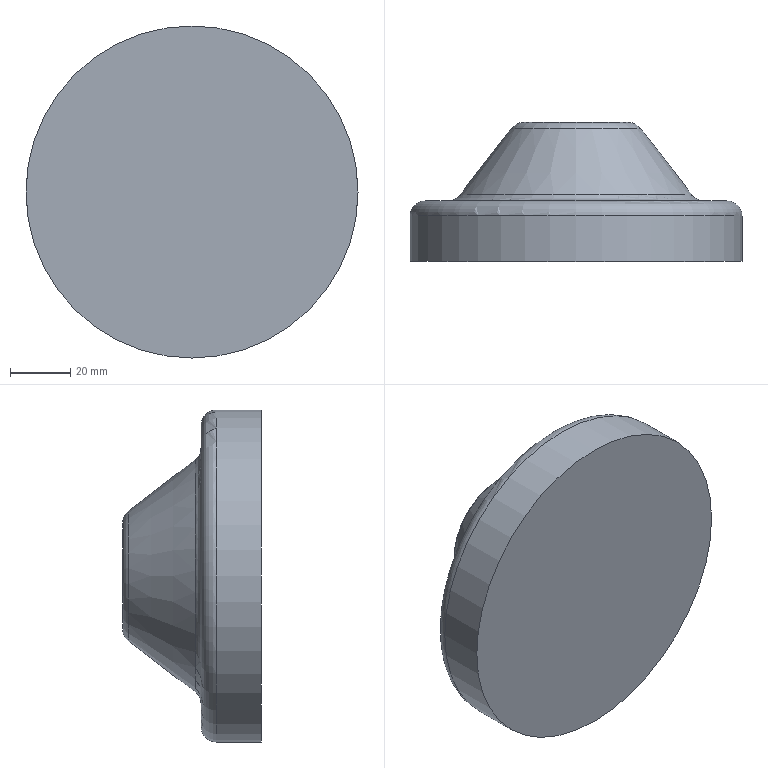Part | STEP file | dijiao | 1 solid | 10 faces | box 110 x 46 x 110 mm | volume 258314 mm3 | plane 4 | torus 3 | cylinder 2 | cone 1 | commonest cylinder face diameters 20 x1 110 x1
STEP:
#1=CARTESIAN_POINT('',(0.,0.,0.));
#2=DIRECTION('',(0.,0.,1.));
#3=DIRECTION('',(1.,0.,0.));
#4=AXIS2_PLACEMENT_3D('',#1,#2,#3);
#5=CARTESIAN_POINT('',(0.,15.,55.));
#6=VERTEX_POINT('',#5);
#7=CARTESIAN_POINT('',(0.,15.,0.));
#8=DIRECTION('',(0.,-1.,0.));
#9=DIRECTION('',(0.,0.,1.));
#10=AXIS2_PLACEMENT_3D('',#7,#8,#9);
#11=CIRCLE('',#10,55.);
#12=CARTESIAN_POINT('',(0.,20.,0.));
#13=DIRECTION('',(0.,-1.,0.));
#14=DIRECTION('',(0.,0.,-1.));
#15=AXIS2_PLACEMENT_3D('',#12,#13,#14);
#16=CYLINDRICAL_SURFACE('',#15,55.);
#17=CARTESIAN_POINT('',(3.142,5.));
#18=DIRECTION('',(1.,0.));
#19=VECTOR('',#18,1.);
#20=LINE('',#17,#19);
#21=(GEOMETRIC_REPRESENTATION_CONTEXT(2)PARAMETRIC_REPRESENTATION_CONTEXT()REPRESENTATION_CONTEXT('',''));
#22=DEFINITIONAL_REPRESENTATION('',(#20),#21);
#23=PCURVE('',#16,#22);
#24=CARTESIAN_POINT('',(0.,15.,0.));
#25=DIRECTION('',(0.,1.,0.));
#26=DIRECTION('',(0.,0.,1.));
#27=AXIS2_PLACEMENT_3D('',#24,#25,#26);
#28=TOROIDAL_SURFACE('',#27,50.,5.);
#29=CARTESIAN_POINT('',(6.283,6.283));
#30=DIRECTION('',(-1.,0.));
#31=VECTOR('',#30,1.);
#32=LINE('',#29,#31);
#33=(GEOMETRIC_REPRESENTATION_CONTEXT(2)PARAMETRIC_REPRESENTATION_CONTEXT()REPRESENTATION_CONTEXT('',''));
#34=DEFINITIONAL_REPRESENTATION('',(#32),#33);
#35=PCURVE('',#28,#34);
#36=SURFACE_CURVE('',#11,(#23,#35),.PCURVE_S1.);
#37=EDGE_CURVE('',#6,#6,#36,.T.);
#38=ORIENTED_EDGE('',*,*,#37,.T.);
#39=CARTESIAN_POINT('',(0.,0.,55.));
#40=VERTEX_POINT('',#39);
#41=CARTESIAN_POINT('',(0.,15.,55.));
#42=CARTESIAN_POINT('',(0.,0.,55.));
#43=B_SPLINE_CURVE_WITH_KNOTS('',1,(#41,#42),.UNSPECIFIED.,.F.,.F.,(2,2),(5.,20.),.PIECEWISE_BEZIER_KNOTS.);
#44=CARTESIAN_POINT('',(9.425,0.));
#45=DIRECTION('',(0.,1.));
#46=VECTOR('',#45,1.);
#47=LINE('',#44,#46);
#48=(GEOMETRIC_REPRESENTATION_CONTEXT(2)PARAMETRIC_REPRESENTATION_CONTEXT()REPRESENTATION_CONTEXT('',''));
#49=DEFINITIONAL_REPRESENTATION('',(#47),#48);
#50=PCURVE('',#16,#49);
#51=CARTESIAN_POINT('',(3.142,0.));
#52=DIRECTION('',(0.,1.));
#53=VECTOR('',#52,1.);
#54=LINE('',#51,#53);
#55=(GEOMETRIC_REPRESENTATION_CONTEXT(2)PARAMETRIC_REPRESENTATION_CONTEXT()REPRESENTATION_CONTEXT('',''));
#56=DEFINITIONAL_REPRESENTATION('',(#54),#55);
#57=PCURVE('',#16,#56);
#58=SEAM_CURVE('',#43,(#50,#57),.PCURVE_S1.);
#59=EDGE_CURVE('',#6,#40,#58,.T.);
#60=ORIENTED_EDGE('',*,*,#59,.T.);
#61=CARTESIAN_POINT('',(0.,0.,0.));
#62=DIRECTION('',(0.,1.,0.));
#63=DIRECTION('',(0.,0.,1.));
#64=AXIS2_PLACEMENT_3D('',#61,#62,#63);
#65=CIRCLE('',#64,55.);
#66=CARTESIAN_POINT('',(9.425,20.));
#67=DIRECTION('',(-1.,0.));
#68=VECTOR('',#67,1.);
#69=LINE('',#66,#68);
#70=(GEOMETRIC_REPRESENTATION_CONTEXT(2)PARAMETRIC_REPRESENTATION_CONTEXT()REPRESENTATION_CONTEXT('',''));
#71=DEFINITIONAL_REPRESENTATION('',(#69),#70);
#72=PCURVE('',#16,#71);
#73=CARTESIAN_POINT('',(0.,0.,0.));
#74=DIRECTION('',(0.,1.,0.));
#75=DIRECTION('',(0.,0.,1.));
#76=AXIS2_PLACEMENT_3D('',#73,#74,#75);
#77=PLANE('',#76);
#78=CARTESIAN_POINT('',(0.,0.));
#79=DIRECTION('',(1.,0.));
#80=AXIS2_PLACEMENT_2D('',#78,#79);
#81=CIRCLE('',#80,55.);
#82=(GEOMETRIC_REPRESENTATION_CONTEXT(2)PARAMETRIC_REPRESENTATION_CONTEXT()REPRESENTATION_CONTEXT('',''));
#83=DEFINITIONAL_REPRESENTATION('',(#81),#82);
#84=PCURVE('',#77,#83);
#85=SURFACE_CURVE('',#65,(#72,#84),.PCURVE_S1.);
#86=EDGE_CURVE('',#40,#40,#85,.T.);
#87=ORIENTED_EDGE('',*,*,#86,.T.);
#88=ORIENTED_EDGE('',*,*,#59,.F.);
#89=EDGE_LOOP('',(#38,#60,#87,#88));
#90=FACE_BOUND('',#89,.T.);
#91=ADVANCED_FACE('',(#90),#16,.T.);
#92=CARTESIAN_POINT('',(0.,20.,42.462));
#93=VERTEX_POINT('',#92);
#94=CARTESIAN_POINT('',(0.,20.,0.));
#95=DIRECTION('',(0.,-1.,0.));
#96=DIRECTION('',(0.,0.,1.));
#97=AXIS2_PLACEMENT_3D('',#94,#95,#96);
#98=CIRCLE('',#97,42.462);
#99=CARTESIAN_POINT('',(0.,20.,0.));
#100=DIRECTION('',(0.,1.,0.));
#101=DIRECTION('',(0.,0.,1.));
#102=AXIS2_PLACEMENT_3D('',#99,#100,#101);
#103=PLANE('',#102);
#104=CARTESIAN_POINT('',(42.462,0.));
#105=CARTESIAN_POINT('',(42.462,-73.546));
#106=CARTESIAN_POINT('',(-21.231,-36.773));
#107=CARTESIAN_POINT('',(-84.924,0.));
#108=CARTESIAN_POINT('',(-21.231,36.773));
#109=CARTESIAN_POINT('',(42.462,73.546));
#110=CARTESIAN_POINT('',(42.462,0.));
#111=(BOUNDED_CURVE()B_SPLINE_CURVE(2,(#104,#105,#106,#107,#108,#109,#110),.UNSPECIFIED.,.T.,.F.)B_SPLINE_CURVE_WITH_KNOTS((1,2,2,2,2,1),(-2.094,0.,2.094,4.189,6.283,8.378),.UNSPECIFIED.)CURVE()GEOMETRIC_REPRESENTATION_ITEM()RATIONAL_B_SPLINE_CURVE((1.,0.5,1.,0.5,1.,0.5,1.))REPRESENTATION_ITEM(''));
#112=(GEOMETRIC_REPRESENTATION_CONTEXT(2)PARAMETRIC_REPRESENTATION_CONTEXT()REPRESENTATION_CONTEXT('',''));
#113=DEFINITIONAL_REPRESENTATION('',(#111),#112);
#114=PCURVE('',#103,#113);
#115=CARTESIAN_POINT('',(0.,25.,0.));
#116=DIRECTION('',(0.,1.,0.));
#117=DIRECTION('',(0.,0.,1.));
#118=AXIS2_PLACEMENT_3D('',#115,#116,#117);
#119=TOROIDAL_SURFACE('',#118,42.462,5.);
#120=CARTESIAN_POINT('',(6.283,4.712));
#121=DIRECTION('',(-1.,0.));
#122=VECTOR('',#121,1.);
#123=LINE('',#120,#122);
#124=(GEOMETRIC_REPRESENTATION_CONTEXT(2)PARAMETRIC_REPRESENTATION_CONTEXT()REPRESENTATION_CONTEXT('',''));
#125=DEFINITIONAL_REPRESENTATION('',(#123),#124);
#126=PCURVE('',#119,#125);
#127=SURFACE_CURVE('',#98,(#114,#126),.PCURVE_S1.);
#128=EDGE_CURVE('',#93,#93,#127,.T.);
#129=ORIENTED_EDGE('',*,*,#128,.T.);
#130=EDGE_LOOP('',(#129));
#131=FACE_BOUND('',#130,.T.);
#132=CARTESIAN_POINT('',(0.,20.,50.));
#133=VERTEX_POINT('',#132);
#134=CARTESIAN_POINT('',(0.,20.,0.));
#135=DIRECTION('',(0.,1.,0.));
#136=DIRECTION('',(0.,0.,1.));
#137=AXIS2_PLACEMENT_3D('',#134,#135,#136);
#138=CIRCLE('',#137,50.);
#139=CARTESIAN_POINT('',(0.,0.));
#140=DIRECTION('',(1.,0.));
#141=AXIS2_PLACEMENT_2D('',#139,#140);
#142=CIRCLE('',#141,50.);
#143=(GEOMETRIC_REPRESENTATION_CONTEXT(2)PARAMETRIC_REPRESENTATION_CONTEXT()REPRESENTATION_CONTEXT('',''));
#144=DEFINITIONAL_REPRESENTATION('',(#142),#143);
#145=PCURVE('',#103,#144);
#146=CARTESIAN_POINT('',(0.,7.854));
#147=DIRECTION('',(1.,0.));
#148=VECTOR('',#147,1.);
#149=LINE('',#146,#148);
#150=(GEOMETRIC_REPRESENTATION_CONTEXT(2)PARAMETRIC_REPRESENTATION_CONTEXT()REPRESENTATION_CONTEXT('',''));
#151=DEFINITIONAL_REPRESENTATION('',(#149),#150);
#152=PCURVE('',#28,#151);
#153=SURFACE_CURVE('',#138,(#145,#152),.PCURVE_S1.);
#154=EDGE_CURVE('',#133,#133,#153,.T.);
#155=ORIENTED_EDGE('',*,*,#154,.T.);
#156=EDGE_LOOP('',(#155));
#157=FACE_BOUND('',#156,.T.);
#158=ADVANCED_FACE('',(#131,#157),#103,.T.);
#159=ORIENTED_EDGE('',*,*,#86,.F.);
#160=EDGE_LOOP('',(#159));
#161=FACE_BOUND('',#160,.T.);
#162=ADVANCED_FACE('',(#161),#77,.F.);
#163=CARTESIAN_POINT('',(0.,21.951,38.499));
#164=VERTEX_POINT('',#163);
#165=CARTESIAN_POINT('',(0.,21.951,0.));
#166=DIRECTION('',(0.,1.,0.));
#167=DIRECTION('',(0.,0.,1.));
#168=AXIS2_PLACEMENT_3D('',#165,#166,#167);
#169=CIRCLE('',#168,38.499);
#170=CARTESIAN_POINT('',(0.,20.,0.));
#171=DIRECTION('',(0.,-1.,0.));
#172=DIRECTION('',(0.,0.,-1.));
#173=AXIS2_PLACEMENT_3D('',#170,#171,#172);
#174=CONICAL_SURFACE('',#173,40.,0.6557);
#175=CARTESIAN_POINT('',(9.425,-1.951));
#176=DIRECTION('',(-1.,0.));
#177=VECTOR('',#176,1.);
#178=LINE('',#175,#177);
#179=(GEOMETRIC_REPRESENTATION_CONTEXT(2)PARAMETRIC_REPRESENTATION_CONTEXT()REPRESENTATION_CONTEXT('',''));
#180=DEFINITIONAL_REPRESENTATION('',(#178),#179);
#181=PCURVE('',#174,#180);
#182=CARTESIAN_POINT('',(0.,3.797));
#183=DIRECTION('',(1.,0.));
#184=VECTOR('',#183,1.);
#185=LINE('',#182,#184);
#186=(GEOMETRIC_REPRESENTATION_CONTEXT(2)PARAMETRIC_REPRESENTATION_CONTEXT()REPRESENTATION_CONTEXT('',''));
#187=DEFINITIONAL_REPRESENTATION('',(#185),#186);
#188=PCURVE('',#119,#187);
#189=SURFACE_CURVE('',#169,(#181,#188),.PCURVE_S1.);
#190=EDGE_CURVE('',#164,#164,#189,.T.);
#191=ORIENTED_EDGE('',*,*,#190,.T.);
#192=CARTESIAN_POINT('',(0.,44.049,21.501));
#193=VERTEX_POINT('',#192);
#194=CARTESIAN_POINT('',(0.,44.049,21.501));
#195=CARTESIAN_POINT('',(0.,21.951,38.499));
#196=B_SPLINE_CURVE_WITH_KNOTS('',1,(#194,#195),.UNSPECIFIED.,.F.,.F.,(2,2),(-30.34,-2.462),.PIECEWISE_BEZIER_KNOTS.);
#197=CARTESIAN_POINT('',(3.142,0.));
#198=DIRECTION('',(0.,1.));
#199=VECTOR('',#198,1.);
#200=LINE('',#197,#199);
#201=(GEOMETRIC_REPRESENTATION_CONTEXT(2)PARAMETRIC_REPRESENTATION_CONTEXT()REPRESENTATION_CONTEXT('',''));
#202=DEFINITIONAL_REPRESENTATION('',(#200),#201);
#203=PCURVE('',#174,#202);
#204=CARTESIAN_POINT('',(9.425,0.));
#205=DIRECTION('',(0.,1.));
#206=VECTOR('',#205,1.);
#207=LINE('',#204,#206);
#208=(GEOMETRIC_REPRESENTATION_CONTEXT(2)PARAMETRIC_REPRESENTATION_CONTEXT()REPRESENTATION_CONTEXT('',''));
#209=DEFINITIONAL_REPRESENTATION('',(#207),#208);
#210=PCURVE('',#174,#209);
#211=SEAM_CURVE('',#196,(#203,#210),.PCURVE_S1.);
#212=EDGE_CURVE('',#193,#164,#211,.T.);
#213=ORIENTED_EDGE('',*,*,#212,.F.);
#214=CARTESIAN_POINT('',(0.,44.049,-21.501));
#215=VERTEX_POINT('',#214);
#216=CARTESIAN_POINT('',(0.,44.049,0.));
#217=DIRECTION('',(0.,-1.,0.));
#218=DIRECTION('',(0.,0.,1.));
#219=AXIS2_PLACEMENT_3D('',#216,#217,#218);
#220=CIRCLE('',#219,21.501);
#221=CARTESIAN_POINT('',(3.142,-24.049));
#222=DIRECTION('',(1.,0.));
#223=VECTOR('',#222,1.);
#224=LINE('',#221,#223);
#225=(GEOMETRIC_REPRESENTATION_CONTEXT(2)PARAMETRIC_REPRESENTATION_CONTEXT()REPRESENTATION_CONTEXT('',''));
#226=DEFINITIONAL_REPRESENTATION('',(#224),#225);
#227=PCURVE('',#174,#226);
#228=CARTESIAN_POINT('',(0.,41.,0.));
#229=DIRECTION('',(0.,-1.,0.));
#230=DIRECTION('',(0.,0.,-1.));
#231=AXIS2_PLACEMENT_3D('',#228,#229,#230);
#232=TOROIDAL_SURFACE('',#231,17.538,5.);
#233=CARTESIAN_POINT('',(3.142,5.627));
#234=DIRECTION('',(1.,0.));
#235=VECTOR('',#234,1.);
#236=LINE('',#233,#235);
#237=(GEOMETRIC_REPRESENTATION_CONTEXT(2)PARAMETRIC_REPRESENTATION_CONTEXT()REPRESENTATION_CONTEXT('',''));
#238=DEFINITIONAL_REPRESENTATION('',(#236),#237);
#239=PCURVE('',#232,#238);
#240=SURFACE_CURVE('',#220,(#227,#239),.PCURVE_S1.);
#241=EDGE_CURVE('',#193,#215,#240,.T.);
#242=ORIENTED_EDGE('',*,*,#241,.T.);
#243=CARTESIAN_POINT('',(0.,44.049,0.));
#244=DIRECTION('',(0.,-1.,0.));
#245=DIRECTION('',(0.,0.,1.));
#246=AXIS2_PLACEMENT_3D('',#243,#244,#245);
#247=CIRCLE('',#246,21.501);
#248=CARTESIAN_POINT('',(3.142,-24.049));
#249=DIRECTION('',(1.,0.));
#250=VECTOR('',#249,1.);
#251=LINE('',#248,#250);
#252=(GEOMETRIC_REPRESENTATION_CONTEXT(2)PARAMETRIC_REPRESENTATION_CONTEXT()REPRESENTATION_CONTEXT('',''));
#253=DEFINITIONAL_REPRESENTATION('',(#251),#252);
#254=PCURVE('',#174,#253);
#255=CARTESIAN_POINT('',(-3.142,5.627));
#256=DIRECTION('',(1.,0.));
#257=VECTOR('',#256,1.);
#258=LINE('',#255,#257);
#259=(GEOMETRIC_REPRESENTATION_CONTEXT(2)PARAMETRIC_REPRESENTATION_CONTEXT()REPRESENTATION_CONTEXT('',''));
#260=DEFINITIONAL_REPRESENTATION('',(#258),#259);
#261=PCURVE('',#232,#260);
#262=SURFACE_CURVE('',#247,(#254,#261),.PCURVE_S1.);
#263=EDGE_CURVE('',#215,#193,#262,.T.);
#264=ORIENTED_EDGE('',*,*,#263,.T.);
#265=ORIENTED_EDGE('',*,*,#212,.T.);
#266=EDGE_LOOP('',(#191,#213,#242,#264,#265));
#267=FACE_BOUND('',#266,.T.);
#268=ADVANCED_FACE('',(#267),#174,.T.);
#269=CARTESIAN_POINT('',(0.,46.,-17.538));
#270=VERTEX_POINT('',#269);
#271=CARTESIAN_POINT('',(0.,46.,0.));
#272=DIRECTION('',(0.,1.,0.));
#273=DIRECTION('',(0.,0.,-1.));
#274=AXIS2_PLACEMENT_3D('',#271,#272,#273);
#275=CIRCLE('',#274,17.538);
#276=CARTESIAN_POINT('',(0.,46.,-20.));
#277=DIRECTION('',(0.,-1.,0.));
#278=DIRECTION('',(0.,0.,-1.));
#279=AXIS2_PLACEMENT_3D('',#276,#277,#278);
#280=PLANE('',#279);
#281=CARTESIAN_POINT('',(-2.462,0.));
#282=CARTESIAN_POINT('',(-2.462,-30.377));
#283=CARTESIAN_POINT('',(-28.769,-15.188));
#284=CARTESIAN_POINT('',(-55.076,0.));
#285=CARTESIAN_POINT('',(-28.769,15.188));
#286=CARTESIAN_POINT('',(-2.462,30.377));
#287=CARTESIAN_POINT('',(-2.462,0.));
#288=(BOUNDED_CURVE()B_SPLINE_CURVE(2,(#281,#282,#283,#284,#285,#286,#287),.UNSPECIFIED.,.T.,.F.)B_SPLINE_CURVE_WITH_KNOTS((1,2,2,2,2,1),(-2.094,0.,2.094,4.189,6.283,8.378),.UNSPECIFIED.)CURVE()GEOMETRIC_REPRESENTATION_ITEM()RATIONAL_B_SPLINE_CURVE((1.,0.5,1.,0.5,1.,0.5,1.))REPRESENTATION_ITEM(''));
#289=(GEOMETRIC_REPRESENTATION_CONTEXT(2)PARAMETRIC_REPRESENTATION_CONTEXT()REPRESENTATION_CONTEXT('',''));
#290=DEFINITIONAL_REPRESENTATION('',(#288),#289);
#291=PCURVE('',#280,#290);
#292=CARTESIAN_POINT('',(6.283,4.712));
#293=DIRECTION('',(-1.,0.));
#294=VECTOR('',#293,1.);
#295=LINE('',#292,#294);
#296=(GEOMETRIC_REPRESENTATION_CONTEXT(2)PARAMETRIC_REPRESENTATION_CONTEXT()REPRESENTATION_CONTEXT('',''));
#297=DEFINITIONAL_REPRESENTATION('',(#295),#296);
#298=PCURVE('',#232,#297);
#299=SURFACE_CURVE('',#275,(#291,#298),.PCURVE_S1.);
#300=EDGE_CURVE('',#270,#270,#299,.T.);
#301=ORIENTED_EDGE('',*,*,#300,.T.);
#302=EDGE_LOOP('',(#301));
#303=FACE_BOUND('',#302,.T.);
#304=CARTESIAN_POINT('',(0.,46.,10.));
#305=VERTEX_POINT('',#304);
#306=CARTESIAN_POINT('',(0.,46.,0.));
#307=DIRECTION('',(0.,1.,0.));
#308=DIRECTION('',(0.,0.,1.));
#309=AXIS2_PLACEMENT_3D('',#306,#307,#308);
#310=CIRCLE('',#309,10.);
#311=CARTESIAN_POINT('',(-30.,0.));
#312=CARTESIAN_POINT('',(-30.,17.321));
#313=CARTESIAN_POINT('',(-15.,8.66));
#314=CARTESIAN_POINT('',(0.,0.));
#315=CARTESIAN_POINT('',(-15.,-8.66));
#316=CARTESIAN_POINT('',(-30.,-17.321));
#317=CARTESIAN_POINT('',(-30.,0.));
#318=(BOUNDED_CURVE()B_SPLINE_CURVE(2,(#311,#312,#313,#314,#315,#316,#317),.UNSPECIFIED.,.T.,.F.)B_SPLINE_CURVE_WITH_KNOTS((1,2,2,2,2,1),(-2.094,0.,2.094,4.189,6.283,8.378),.UNSPECIFIED.)CURVE()GEOMETRIC_REPRESENTATION_ITEM()RATIONAL_B_SPLINE_CURVE((1.,0.5,1.,0.5,1.,0.5,1.))REPRESENTATION_ITEM(''));
#319=(GEOMETRIC_REPRESENTATION_CONTEXT(2)PARAMETRIC_REPRESENTATION_CONTEXT()REPRESENTATION_CONTEXT('',''));
#320=DEFINITIONAL_REPRESENTATION('',(#318),#319);
#321=PCURVE('',#280,#320);
#322=CARTESIAN_POINT('',(0.,26.,0.));
#323=DIRECTION('',(0.,1.,0.));
#324=DIRECTION('',(0.,0.,1.));
#325=AXIS2_PLACEMENT_3D('',#322,#323,#324);
#326=CYLINDRICAL_SURFACE('',#325,10.);
#327=CARTESIAN_POINT('',(0.,20.));
#328=DIRECTION('',(1.,0.));
#329=VECTOR('',#328,1.);
#330=LINE('',#327,#329);
#331=(GEOMETRIC_REPRESENTATION_CONTEXT(2)PARAMETRIC_REPRESENTATION_CONTEXT()REPRESENTATION_CONTEXT('',''));
#332=DEFINITIONAL_REPRESENTATION('',(#330),#331);
#333=PCURVE('',#326,#332);
#334=SURFACE_CURVE('',#310,(#321,#333),.PCURVE_S1.);
#335=EDGE_CURVE('',#305,#305,#334,.T.);
#336=ORIENTED_EDGE('',*,*,#335,.F.);
#337=EDGE_LOOP('',(#336));
#338=FACE_BOUND('',#337,.T.);
#339=ADVANCED_FACE('',(#303,#338),#280,.F.);
#340=CARTESIAN_POINT('',(0.,26.,10.));
#341=VERTEX_POINT('',#340);
#342=CARTESIAN_POINT('',(0.,26.,0.));
#343=DIRECTION('',(0.,1.,0.));
#344=DIRECTION('',(0.,0.,1.));
#345=AXIS2_PLACEMENT_3D('',#342,#343,#344);
#346=CIRCLE('',#345,10.);
#347=CARTESIAN_POINT('',(0.,0.));
#348=DIRECTION('',(1.,0.));
#349=VECTOR('',#348,1.);
#350=LINE('',#347,#349);
#351=(GEOMETRIC_REPRESENTATION_CONTEXT(2)PARAMETRIC_REPRESENTATION_CONTEXT()REPRESENTATION_CONTEXT('',''));
#352=DEFINITIONAL_REPRESENTATION('',(#350),#351);
#353=PCURVE('',#326,#352);
#354=CARTESIAN_POINT('',(0.,26.,0.));
#355=DIRECTION('',(0.,1.,0.));
#356=DIRECTION('',(0.,0.,1.));
#357=AXIS2_PLACEMENT_3D('',#354,#355,#356);
#358=PLANE('',#357);
#359=CARTESIAN_POINT('',(0.,0.));
#360=DIRECTION('',(1.,0.));
#361=AXIS2_PLACEMENT_2D('',#359,#360);
#362=CIRCLE('',#361,10.);
#363=(GEOMETRIC_REPRESENTATION_CONTEXT(2)PARAMETRIC_REPRESENTATION_CONTEXT()REPRESENTATION_CONTEXT('',''));
#364=DEFINITIONAL_REPRESENTATION('',(#362),#363);
#365=PCURVE('',#358,#364);
#366=SURFACE_CURVE('',#346,(#353,#365),.PCURVE_S1.);
#367=EDGE_CURVE('',#341,#341,#366,.T.);
#368=ORIENTED_EDGE('',*,*,#367,.T.);
#369=CARTESIAN_POINT('',(0.,26.,10.));
#370=CARTESIAN_POINT('',(0.,46.,10.));
#371=B_SPLINE_CURVE_WITH_KNOTS('',1,(#369,#370),.UNSPECIFIED.,.F.,.F.,(2,2),(0.,20.),.PIECEWISE_BEZIER_KNOTS.);
#372=CARTESIAN_POINT('',(6.283,0.));
#373=DIRECTION('',(0.,1.));
#374=VECTOR('',#373,1.);
#375=LINE('',#372,#374);
#376=(GEOMETRIC_REPRESENTATION_CONTEXT(2)PARAMETRIC_REPRESENTATION_CONTEXT()REPRESENTATION_CONTEXT('',''));
#377=DEFINITIONAL_REPRESENTATION('',(#375),#376);
#378=PCURVE('',#326,#377);
#379=CARTESIAN_POINT('',(0.,0.));
#380=DIRECTION('',(0.,1.));
#381=VECTOR('',#380,1.);
#382=LINE('',#379,#381);
#383=(GEOMETRIC_REPRESENTATION_CONTEXT(2)PARAMETRIC_REPRESENTATION_CONTEXT()REPRESENTATION_CONTEXT('',''));
#384=DEFINITIONAL_REPRESENTATION('',(#382),#383);
#385=PCURVE('',#326,#384);
#386=SEAM_CURVE('',#371,(#378,#385),.PCURVE_S1.);
#387=EDGE_CURVE('',#341,#305,#386,.T.);
#388=ORIENTED_EDGE('',*,*,#387,.T.);
#389=ORIENTED_EDGE('',*,*,#335,.F.);
#390=ORIENTED_EDGE('',*,*,#387,.F.);
#391=EDGE_LOOP('',(#368,#388,#389,#390));
#392=FACE_BOUND('',#391,.F.);
#393=ADVANCED_FACE('',(#392),#326,.F.);
#394=ORIENTED_EDGE('',*,*,#367,.T.);
#395=EDGE_LOOP('',(#394));
#396=FACE_BOUND('',#395,.T.);
#397=ADVANCED_FACE('',(#396),#358,.T.);
#398=ORIENTED_EDGE('',*,*,#37,.F.);
#399=CARTESIAN_POINT('',(0.,15.,55.));
#400=CARTESIAN_POINT('',(0.,16.337,55.));
#401=CARTESIAN_POINT('',(0.,17.639,54.575));
#402=CARTESIAN_POINT('',(0.,18.76,53.76));
#403=CARTESIAN_POINT('',(0.,19.575,52.639));
#404=CARTESIAN_POINT('',(0.,20.,51.337));
#405=CARTESIAN_POINT('',(0.,20.,50.));
#406=(BOUNDED_CURVE()B_SPLINE_CURVE(6,(#399,#400,#401,#402,#403,#404,#405),.UNSPECIFIED.,.F.,.F.)B_SPLINE_CURVE_WITH_KNOTS((7,7),(0.,1.571),.PIECEWISE_BEZIER_KNOTS.)CURVE()GEOMETRIC_REPRESENTATION_ITEM()RATIONAL_B_SPLINE_CURVE((1.031,1.01,0.9979,0.994,0.9979,1.01,1.031))REPRESENTATION_ITEM(''));
#407=CARTESIAN_POINT('',(6.283,6.283));
#408=DIRECTION('',(0.,1.));
#409=VECTOR('',#408,1.);
#410=LINE('',#407,#409);
#411=(GEOMETRIC_REPRESENTATION_CONTEXT(2)PARAMETRIC_REPRESENTATION_CONTEXT()REPRESENTATION_CONTEXT('',''));
#412=DEFINITIONAL_REPRESENTATION('',(#410),#411);
#413=PCURVE('',#28,#412);
#414=CARTESIAN_POINT('',(0.,6.283));
#415=DIRECTION('',(0.,1.));
#416=VECTOR('',#415,1.);
#417=LINE('',#414,#416);
#418=(GEOMETRIC_REPRESENTATION_CONTEXT(2)PARAMETRIC_REPRESENTATION_CONTEXT()REPRESENTATION_CONTEXT('',''));
#419=DEFINITIONAL_REPRESENTATION('',(#417),#418);
#420=PCURVE('',#28,#419);
#421=SEAM_CURVE('',#406,(#413,#420),.PCURVE_S1.);
#422=EDGE_CURVE('',#6,#133,#421,.T.);
#423=ORIENTED_EDGE('',*,*,#422,.T.);
#424=ORIENTED_EDGE('',*,*,#154,.F.);
#425=ORIENTED_EDGE('',*,*,#422,.F.);
#426=EDGE_LOOP('',(#398,#423,#424,#425));
#427=FACE_BOUND('',#426,.T.);
#428=ADVANCED_FACE('',(#427),#28,.T.);
#429=ORIENTED_EDGE('',*,*,#263,.F.);
#430=CARTESIAN_POINT('',(0.,46.,-17.538));
#431=CARTESIAN_POINT('',(0.,46.,-18.306));
#432=CARTESIAN_POINT('',(0.,45.859,-19.067));
#433=CARTESIAN_POINT('',(0.,45.58,-19.793));
#434=CARTESIAN_POINT('',(0.,45.175,-20.457));
#435=CARTESIAN_POINT('',(0.,44.657,-21.033));
#436=CARTESIAN_POINT('',(0.,44.049,-21.501));
#437=(BOUNDED_CURVE()B_SPLINE_CURVE(6,(#430,#431,#432,#433,#434,#435,#436),.UNSPECIFIED.,.F.,.F.)B_SPLINE_CURVE_WITH_KNOTS((7,7),(4.712,5.627),.PIECEWISE_BEZIER_KNOTS.)CURVE()GEOMETRIC_REPRESENTATION_ITEM()RATIONAL_B_SPLINE_CURVE((1.011,1.003,0.9993,0.9979,0.9993,1.003,1.011))REPRESENTATION_ITEM(''));
#438=CARTESIAN_POINT('',(0.,0.));
#439=DIRECTION('',(0.,1.));
#440=VECTOR('',#439,1.);
#441=LINE('',#438,#440);
#442=(GEOMETRIC_REPRESENTATION_CONTEXT(2)PARAMETRIC_REPRESENTATION_CONTEXT()REPRESENTATION_CONTEXT('',''));
#443=DEFINITIONAL_REPRESENTATION('',(#441),#442);
#444=PCURVE('',#232,#443);
#445=CARTESIAN_POINT('',(6.283,0.));
#446=DIRECTION('',(0.,1.));
#447=VECTOR('',#446,1.);
#448=LINE('',#445,#447);
#449=(GEOMETRIC_REPRESENTATION_CONTEXT(2)PARAMETRIC_REPRESENTATION_CONTEXT()REPRESENTATION_CONTEXT('',''));
#450=DEFINITIONAL_REPRESENTATION('',(#448),#449);
#451=PCURVE('',#232,#450);
#452=SEAM_CURVE('',#437,(#444,#451),.PCURVE_S1.);
#453=EDGE_CURVE('',#270,#215,#452,.T.);
#454=ORIENTED_EDGE('',*,*,#453,.F.);
#455=ORIENTED_EDGE('',*,*,#300,.F.);
#456=ORIENTED_EDGE('',*,*,#453,.T.);
#457=ORIENTED_EDGE('',*,*,#241,.F.);
#458=EDGE_LOOP('',(#429,#454,#455,#456,#457));
#459=FACE_BOUND('',#458,.T.);
#460=ADVANCED_FACE('',(#459),#232,.T.);
#461=ORIENTED_EDGE('',*,*,#128,.T.);
#462=CARTESIAN_POINT('',(0.,21.951,38.499));
#463=CARTESIAN_POINT('',(0.,21.343,38.967));
#464=CARTESIAN_POINT('',(0.,20.825,39.543));
#465=CARTESIAN_POINT('',(0.,20.42,40.207));
#466=CARTESIAN_POINT('',(0.,20.141,40.933));
#467=CARTESIAN_POINT('',(0.,20.,41.694));
#468=CARTESIAN_POINT('',(0.,20.,42.462));
#469=(BOUNDED_CURVE()B_SPLINE_CURVE(6,(#462,#463,#464,#465,#466,#467,#468),.UNSPECIFIED.,.F.,.F.)B_SPLINE_CURVE_WITH_KNOTS((7,7),(3.797,4.712),.PIECEWISE_BEZIER_KNOTS.)CURVE()GEOMETRIC_REPRESENTATION_ITEM()RATIONAL_B_SPLINE_CURVE((1.011,1.003,0.9993,0.9979,0.9993,1.003,1.011))REPRESENTATION_ITEM(''));
#470=CARTESIAN_POINT('',(0.,0.));
#471=DIRECTION('',(0.,1.));
#472=VECTOR('',#471,1.);
#473=LINE('',#470,#472);
#474=(GEOMETRIC_REPRESENTATION_CONTEXT(2)PARAMETRIC_REPRESENTATION_CONTEXT()REPRESENTATION_CONTEXT('',''));
#475=DEFINITIONAL_REPRESENTATION('',(#473),#474);
#476=PCURVE('',#119,#475);
#477=CARTESIAN_POINT('',(6.283,0.));
#478=DIRECTION('',(0.,1.));
#479=VECTOR('',#478,1.);
#480=LINE('',#477,#479);
#481=(GEOMETRIC_REPRESENTATION_CONTEXT(2)PARAMETRIC_REPRESENTATION_CONTEXT()REPRESENTATION_CONTEXT('',''));
#482=DEFINITIONAL_REPRESENTATION('',(#480),#481);
#483=PCURVE('',#119,#482);
#484=SEAM_CURVE('',#469,(#476,#483),.PCURVE_S1.);
#485=EDGE_CURVE('',#164,#93,#484,.T.);
#486=ORIENTED_EDGE('',*,*,#485,.F.);
#487=ORIENTED_EDGE('',*,*,#190,.T.);
#488=ORIENTED_EDGE('',*,*,#485,.T.);
#489=EDGE_LOOP('',(#461,#486,#487,#488));
#490=FACE_BOUND('',#489,.F.);
#491=ADVANCED_FACE('',(#490),#119,.F.);
#492=CLOSED_SHELL('',(#91,#158,#162,#268,#339,#393,#397,#428,#460,#491));
#493=MANIFOLD_SOLID_BREP('',#492);
#494=(LENGTH_UNIT()NAMED_UNIT(*)SI_UNIT(.MILLI.,.METRE.));
#495=UNCERTAINTY_MEASURE_WITH_UNIT(LENGTH_MEASURE(0.00001),#494,'','');
#496=(NAMED_UNIT(*)PLANE_ANGLE_UNIT()SI_UNIT($,.RADIAN.));
#497=(NAMED_UNIT(*)SI_UNIT($,.STERADIAN.)SOLID_ANGLE_UNIT());
#498=(GEOMETRIC_REPRESENTATION_CONTEXT(3)GLOBAL_UNCERTAINTY_ASSIGNED_CONTEXT((#495))GLOBAL_UNIT_ASSIGNED_CONTEXT((#494,#496,#497))REPRESENTATION_CONTEXT('',''));
#499=ADVANCED_BREP_SHAPE_REPRESENTATION('',(#4,#493),#498);